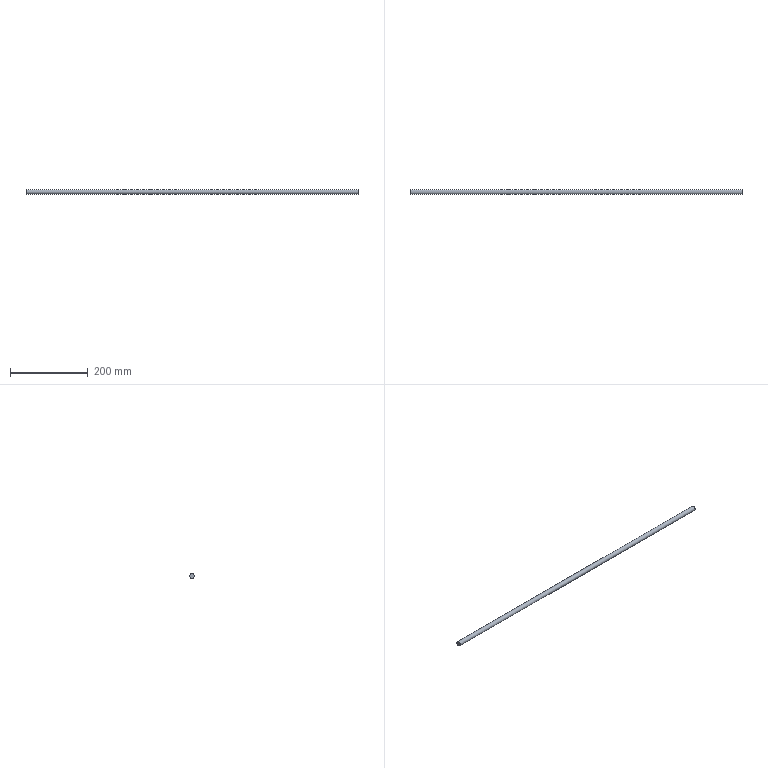Part | STEP file | solid 192 | 1 solid | 3 faces | box 855 x 12 x 12 mm | volume 96698 mm3 | plane 2 | cylinder 1 | commonest cylinder face diameters 12 x1